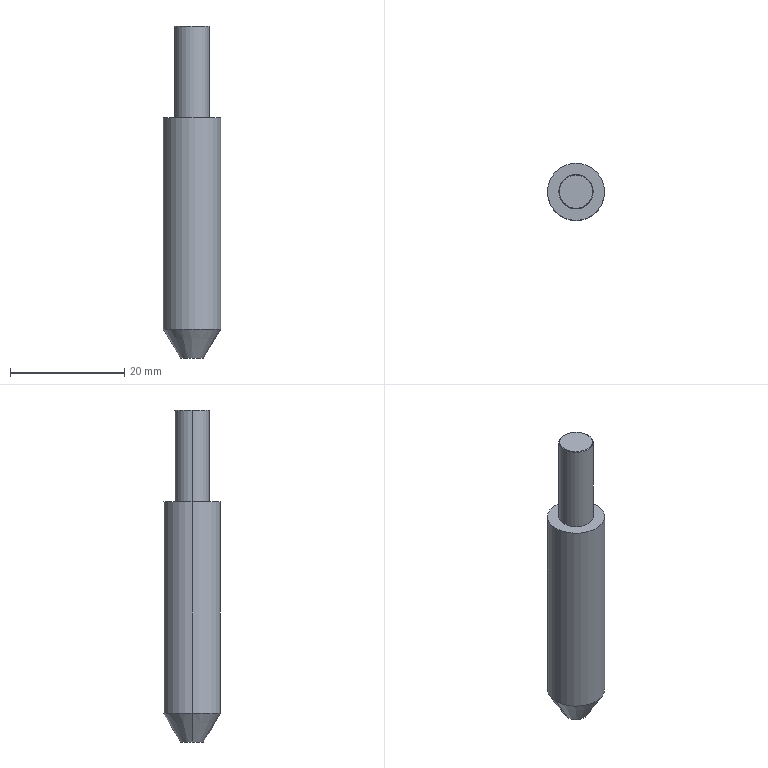Part | STEP file | Pin | 1 solid | 11 faces | box 10 x 10 x 58 mm | volume 3562 mm3 | cone 4 | cylinder 4 | plane 3 | commonest cylinder face diameters 6 x2 10 x2
STEP:
#1=CARTESIAN_POINT('',(0.,0.,0.));
#2=DIRECTION('',(0.,0.,1.));
#3=DIRECTION('',(1.,0.,0.));
#4=AXIS2_PLACEMENT_3D('',#1,#2,#3);
#5=CARTESIAN_POINT('',(-2.,0.,0.));
#6=VERTEX_POINT('',#5);
#7=CARTESIAN_POINT('',(2.,0.,0.));
#8=VERTEX_POINT('',#7);
#9=CARTESIAN_POINT('',(0.,0.,0.));
#10=DIRECTION('',(0.,0.,-1.));
#11=DIRECTION('',(1.,0.,0.));
#12=AXIS2_PLACEMENT_3D('',#9,#10,#11);
#13=CIRCLE('',#12,2.);
#14=CARTESIAN_POINT('',(0.,0.,5.));
#15=DIRECTION('',(0.,0.,1.));
#16=DIRECTION('',(1.,0.,0.));
#17=AXIS2_PLACEMENT_3D('',#14,#15,#16);
#18=CONICAL_SURFACE('',#17,5.,0.5404);
#19=CARTESIAN_POINT('',(6.283,-5.));
#20=DIRECTION('',(-1.,0.));
#21=VECTOR('',#20,1.);
#22=LINE('',#19,#21);
#23=(GEOMETRIC_REPRESENTATION_CONTEXT(2)PARAMETRIC_REPRESENTATION_CONTEXT()REPRESENTATION_CONTEXT('',''));
#24=DEFINITIONAL_REPRESENTATION('',(#22),#23);
#25=PCURVE('',#18,#24);
#26=CARTESIAN_POINT('',(0.,0.,0.));
#27=DIRECTION('',(0.,0.,1.));
#28=DIRECTION('',(1.,0.,0.));
#29=AXIS2_PLACEMENT_3D('',#26,#27,#28);
#30=PLANE('',#29);
#31=CARTESIAN_POINT('',(2.,0.));
#32=CARTESIAN_POINT('',(2.,-3.464));
#33=CARTESIAN_POINT('',(-1.,-1.732));
#34=CARTESIAN_POINT('',(-4.,0.));
#35=CARTESIAN_POINT('',(-1.,1.732));
#36=CARTESIAN_POINT('',(2.,3.464));
#37=CARTESIAN_POINT('',(2.,0.));
#38=(BOUNDED_CURVE()B_SPLINE_CURVE(2,(#31,#32,#33,#34,#35,#36,#37),.UNSPECIFIED.,.T.,.F.)B_SPLINE_CURVE_WITH_KNOTS((1,2,2,2,2,1),(-2.094,0.,2.094,4.189,6.283,8.378),.UNSPECIFIED.)CURVE()GEOMETRIC_REPRESENTATION_ITEM()RATIONAL_B_SPLINE_CURVE((1.,0.5,1.,0.5,1.,0.5,1.))REPRESENTATION_ITEM(''));
#39=(GEOMETRIC_REPRESENTATION_CONTEXT(2)PARAMETRIC_REPRESENTATION_CONTEXT()REPRESENTATION_CONTEXT('',''));
#40=DEFINITIONAL_REPRESENTATION('',(#38),#39);
#41=PCURVE('',#30,#40);
#42=SURFACE_CURVE('',#13,(#25,#41),.PCURVE_S1.);
#43=EDGE_CURVE('',#6,#8,#42,.T.);
#44=ORIENTED_EDGE('',*,*,#43,.F.);
#45=CARTESIAN_POINT('',(-5.,0.,5.));
#46=VERTEX_POINT('',#45);
#47=CARTESIAN_POINT('',(-5.,0.,5.));
#48=DIRECTION('',(-0.5145,0.,0.8575));
#49=VECTOR('',#48,1.);
#50=LINE('',#47,#49);
#51=CARTESIAN_POINT('',(3.142,0.));
#52=DIRECTION('',(0.,1.));
#53=VECTOR('',#52,1.);
#54=LINE('',#51,#53);
#55=(GEOMETRIC_REPRESENTATION_CONTEXT(2)PARAMETRIC_REPRESENTATION_CONTEXT()REPRESENTATION_CONTEXT('',''));
#56=DEFINITIONAL_REPRESENTATION('',(#54),#55);
#57=PCURVE('',#18,#56);
#58=CARTESIAN_POINT('',(0.,0.,5.));
#59=DIRECTION('',(0.,0.,1.));
#60=DIRECTION('',(1.,0.,0.));
#61=AXIS2_PLACEMENT_3D('',#58,#59,#60);
#62=CONICAL_SURFACE('',#61,5.,0.5404);
#63=CARTESIAN_POINT('',(3.142,0.));
#64=DIRECTION('',(0.,1.));
#65=VECTOR('',#64,1.);
#66=LINE('',#63,#65);
#67=(GEOMETRIC_REPRESENTATION_CONTEXT(2)PARAMETRIC_REPRESENTATION_CONTEXT()REPRESENTATION_CONTEXT('',''));
#68=DEFINITIONAL_REPRESENTATION('',(#66),#67);
#69=PCURVE('',#62,#68);
#70=SURFACE_CURVE('',#50,(#57,#69),.PCURVE_S1.);
#71=EDGE_CURVE('',#6,#46,#70,.T.);
#72=ORIENTED_EDGE('',*,*,#71,.T.);
#73=CARTESIAN_POINT('',(5.,0.,5.));
#74=VERTEX_POINT('',#73);
#75=CARTESIAN_POINT('',(0.,0.,5.));
#76=DIRECTION('',(0.,0.,1.));
#77=DIRECTION('',(1.,0.,0.));
#78=AXIS2_PLACEMENT_3D('',#75,#76,#77);
#79=CIRCLE('',#78,5.);
#80=CARTESIAN_POINT('',(0.,0.));
#81=DIRECTION('',(1.,0.));
#82=VECTOR('',#81,1.);
#83=LINE('',#80,#82);
#84=(GEOMETRIC_REPRESENTATION_CONTEXT(2)PARAMETRIC_REPRESENTATION_CONTEXT()REPRESENTATION_CONTEXT('',''));
#85=DEFINITIONAL_REPRESENTATION('',(#83),#84);
#86=PCURVE('',#18,#85);
#87=CARTESIAN_POINT('',(0.,0.,42.));
#88=DIRECTION('',(0.,0.,-1.));
#89=DIRECTION('',(-1.,0.,0.));
#90=AXIS2_PLACEMENT_3D('',#87,#88,#89);
#91=CYLINDRICAL_SURFACE('',#90,5.);
#92=CARTESIAN_POINT('',(3.142,37.));
#93=DIRECTION('',(-1.,0.));
#94=VECTOR('',#93,1.);
#95=LINE('',#92,#94);
#96=(GEOMETRIC_REPRESENTATION_CONTEXT(2)PARAMETRIC_REPRESENTATION_CONTEXT()REPRESENTATION_CONTEXT('',''));
#97=DEFINITIONAL_REPRESENTATION('',(#95),#96);
#98=PCURVE('',#91,#97);
#99=SURFACE_CURVE('',#79,(#86,#98),.PCURVE_S1.);
#100=EDGE_CURVE('',#74,#46,#99,.T.);
#101=ORIENTED_EDGE('',*,*,#100,.F.);
#102=CARTESIAN_POINT('',(5.,0.,5.));
#103=DIRECTION('',(0.5145,0.,0.8575));
#104=VECTOR('',#103,1.);
#105=LINE('',#102,#104);
#106=CARTESIAN_POINT('',(0.,0.));
#107=DIRECTION('',(0.,1.));
#108=VECTOR('',#107,1.);
#109=LINE('',#106,#108);
#110=(GEOMETRIC_REPRESENTATION_CONTEXT(2)PARAMETRIC_REPRESENTATION_CONTEXT()REPRESENTATION_CONTEXT('',''));
#111=DEFINITIONAL_REPRESENTATION('',(#109),#110);
#112=PCURVE('',#18,#111);
#113=CARTESIAN_POINT('',(6.283,0.));
#114=DIRECTION('',(0.,1.));
#115=VECTOR('',#114,1.);
#116=LINE('',#113,#115);
#117=(GEOMETRIC_REPRESENTATION_CONTEXT(2)PARAMETRIC_REPRESENTATION_CONTEXT()REPRESENTATION_CONTEXT('',''));
#118=DEFINITIONAL_REPRESENTATION('',(#116),#117);
#119=PCURVE('',#62,#118);
#120=SURFACE_CURVE('',#105,(#112,#119),.PCURVE_S1.);
#121=EDGE_CURVE('',#8,#74,#120,.T.);
#122=ORIENTED_EDGE('',*,*,#121,.F.);
#123=EDGE_LOOP('',(#44,#72,#101,#122));
#124=FACE_BOUND('',#123,.T.);
#125=ADVANCED_FACE('',(#124),#18,.T.);
#126=CARTESIAN_POINT('',(2.9,0.,58.));
#127=VERTEX_POINT('',#126);
#128=CARTESIAN_POINT('',(-2.9,0.,58.));
#129=VERTEX_POINT('',#128);
#130=CARTESIAN_POINT('',(0.,0.,58.));
#131=DIRECTION('',(0.,0.,1.));
#132=DIRECTION('',(1.,0.,0.));
#133=AXIS2_PLACEMENT_3D('',#130,#131,#132);
#134=CIRCLE('',#133,2.9);
#135=CARTESIAN_POINT('',(0.,0.,58.));
#136=DIRECTION('',(0.,0.,-1.));
#137=DIRECTION('',(-1.,0.,0.));
#138=AXIS2_PLACEMENT_3D('',#135,#136,#137);
#139=CONICAL_SURFACE('',#138,2.9,0.7854);
#140=CARTESIAN_POINT('',(3.142,0.));
#141=DIRECTION('',(-1.,0.));
#142=VECTOR('',#141,1.);
#143=LINE('',#140,#142);
#144=(GEOMETRIC_REPRESENTATION_CONTEXT(2)PARAMETRIC_REPRESENTATION_CONTEXT()REPRESENTATION_CONTEXT('',''));
#145=DEFINITIONAL_REPRESENTATION('',(#143),#144);
#146=PCURVE('',#139,#145);
#147=CARTESIAN_POINT('',(0.,0.,58.));
#148=DIRECTION('',(0.,0.,1.));
#149=DIRECTION('',(1.,0.,0.));
#150=AXIS2_PLACEMENT_3D('',#147,#148,#149);
#151=PLANE('',#150);
#152=CARTESIAN_POINT('',(0.,0.));
#153=DIRECTION('',(1.,0.));
#154=AXIS2_PLACEMENT_2D('',#152,#153);
#155=CIRCLE('',#154,2.9);
#156=(GEOMETRIC_REPRESENTATION_CONTEXT(2)PARAMETRIC_REPRESENTATION_CONTEXT()REPRESENTATION_CONTEXT('',''));
#157=DEFINITIONAL_REPRESENTATION('',(#155),#156);
#158=PCURVE('',#151,#157);
#159=SURFACE_CURVE('',#134,(#146,#158),.PCURVE_S1.);
#160=EDGE_CURVE('',#127,#129,#159,.T.);
#161=ORIENTED_EDGE('',*,*,#160,.F.);
#162=CARTESIAN_POINT('',(3.,0.,57.9));
#163=VERTEX_POINT('',#162);
#164=CARTESIAN_POINT('',(2.9,0.,58.));
#165=DIRECTION('',(0.7071,0.,-0.7071));
#166=VECTOR('',#165,1.);
#167=LINE('',#164,#166);
#168=CARTESIAN_POINT('',(3.142,0.));
#169=DIRECTION('',(0.,1.));
#170=VECTOR('',#169,1.);
#171=LINE('',#168,#170);
#172=(GEOMETRIC_REPRESENTATION_CONTEXT(2)PARAMETRIC_REPRESENTATION_CONTEXT()REPRESENTATION_CONTEXT('',''));
#173=DEFINITIONAL_REPRESENTATION('',(#171),#172);
#174=PCURVE('',#139,#173);
#175=CARTESIAN_POINT('',(0.,0.,58.));
#176=DIRECTION('',(0.,0.,-1.));
#177=DIRECTION('',(-1.,0.,0.));
#178=AXIS2_PLACEMENT_3D('',#175,#176,#177);
#179=CONICAL_SURFACE('',#178,2.9,0.7854);
#180=CARTESIAN_POINT('',(3.142,0.));
#181=DIRECTION('',(0.,1.));
#182=VECTOR('',#181,1.);
#183=LINE('',#180,#182);
#184=(GEOMETRIC_REPRESENTATION_CONTEXT(2)PARAMETRIC_REPRESENTATION_CONTEXT()REPRESENTATION_CONTEXT('',''));
#185=DEFINITIONAL_REPRESENTATION('',(#183),#184);
#186=PCURVE('',#179,#185);
#187=SURFACE_CURVE('',#167,(#174,#186),.PCURVE_S1.);
#188=EDGE_CURVE('',#127,#163,#187,.T.);
#189=ORIENTED_EDGE('',*,*,#188,.T.);
#190=CARTESIAN_POINT('',(-3.,0.,57.9));
#191=VERTEX_POINT('',#190);
#192=CARTESIAN_POINT('',(0.,0.,57.9));
#193=DIRECTION('',(0.,0.,-1.));
#194=DIRECTION('',(1.,0.,0.));
#195=AXIS2_PLACEMENT_3D('',#192,#193,#194);
#196=CIRCLE('',#195,3.);
#197=CARTESIAN_POINT('',(-3.142,0.1));
#198=DIRECTION('',(1.,0.));
#199=VECTOR('',#198,1.);
#200=LINE('',#197,#199);
#201=(GEOMETRIC_REPRESENTATION_CONTEXT(2)PARAMETRIC_REPRESENTATION_CONTEXT()REPRESENTATION_CONTEXT('',''));
#202=DEFINITIONAL_REPRESENTATION('',(#200),#201);
#203=PCURVE('',#139,#202);
#204=CARTESIAN_POINT('',(0.,0.,58.));
#205=DIRECTION('',(0.,0.,-1.));
#206=DIRECTION('',(-1.,0.,0.));
#207=AXIS2_PLACEMENT_3D('',#204,#205,#206);
#208=CYLINDRICAL_SURFACE('',#207,3.);
#209=CARTESIAN_POINT('',(-3.142,0.1));
#210=DIRECTION('',(1.,0.));
#211=VECTOR('',#210,1.);
#212=LINE('',#209,#211);
#213=(GEOMETRIC_REPRESENTATION_CONTEXT(2)PARAMETRIC_REPRESENTATION_CONTEXT()REPRESENTATION_CONTEXT('',''));
#214=DEFINITIONAL_REPRESENTATION('',(#212),#213);
#215=PCURVE('',#208,#214);
#216=SURFACE_CURVE('',#196,(#203,#215),.PCURVE_S1.);
#217=EDGE_CURVE('',#191,#163,#216,.T.);
#218=ORIENTED_EDGE('',*,*,#217,.F.);
#219=CARTESIAN_POINT('',(-2.9,0.,58.));
#220=DIRECTION('',(-0.7071,0.,-0.7071));
#221=VECTOR('',#220,1.);
#222=LINE('',#219,#221);
#223=CARTESIAN_POINT('',(0.,0.));
#224=DIRECTION('',(0.,1.));
#225=VECTOR('',#224,1.);
#226=LINE('',#223,#225);
#227=(GEOMETRIC_REPRESENTATION_CONTEXT(2)PARAMETRIC_REPRESENTATION_CONTEXT()REPRESENTATION_CONTEXT('',''));
#228=DEFINITIONAL_REPRESENTATION('',(#226),#227);
#229=PCURVE('',#139,#228);
#230=CARTESIAN_POINT('',(6.283,0.));
#231=DIRECTION('',(0.,1.));
#232=VECTOR('',#231,1.);
#233=LINE('',#230,#232);
#234=(GEOMETRIC_REPRESENTATION_CONTEXT(2)PARAMETRIC_REPRESENTATION_CONTEXT()REPRESENTATION_CONTEXT('',''));
#235=DEFINITIONAL_REPRESENTATION('',(#233),#234);
#236=PCURVE('',#179,#235);
#237=SURFACE_CURVE('',#222,(#229,#236),.PCURVE_S1.);
#238=EDGE_CURVE('',#129,#191,#237,.T.);
#239=ORIENTED_EDGE('',*,*,#238,.F.);
#240=EDGE_LOOP('',(#161,#189,#218,#239));
#241=FACE_BOUND('',#240,.T.);
#242=ADVANCED_FACE('',(#241),#139,.T.);
#243=ORIENTED_EDGE('',*,*,#217,.T.);
#244=CARTESIAN_POINT('',(3.,0.,42.));
#245=VERTEX_POINT('',#244);
#246=CARTESIAN_POINT('',(3.,0.,58.));
#247=DIRECTION('',(0.,0.,-1.));
#248=VECTOR('',#247,1.);
#249=LINE('',#246,#248);
#250=CARTESIAN_POINT('',(3.142,0.));
#251=DIRECTION('',(0.,1.));
#252=VECTOR('',#251,1.);
#253=LINE('',#250,#252);
#254=(GEOMETRIC_REPRESENTATION_CONTEXT(2)PARAMETRIC_REPRESENTATION_CONTEXT()REPRESENTATION_CONTEXT('',''));
#255=DEFINITIONAL_REPRESENTATION('',(#253),#254);
#256=PCURVE('',#208,#255);
#257=CARTESIAN_POINT('',(0.,0.,58.));
#258=DIRECTION('',(0.,0.,-1.));
#259=DIRECTION('',(-1.,0.,0.));
#260=AXIS2_PLACEMENT_3D('',#257,#258,#259);
#261=CYLINDRICAL_SURFACE('',#260,3.);
#262=CARTESIAN_POINT('',(3.142,0.));
#263=DIRECTION('',(0.,1.));
#264=VECTOR('',#263,1.);
#265=LINE('',#262,#264);
#266=(GEOMETRIC_REPRESENTATION_CONTEXT(2)PARAMETRIC_REPRESENTATION_CONTEXT()REPRESENTATION_CONTEXT('',''));
#267=DEFINITIONAL_REPRESENTATION('',(#265),#266);
#268=PCURVE('',#261,#267);
#269=SURFACE_CURVE('',#249,(#256,#268),.PCURVE_S1.);
#270=EDGE_CURVE('',#163,#245,#269,.T.);
#271=ORIENTED_EDGE('',*,*,#270,.T.);
#272=CARTESIAN_POINT('',(-3.,0.,42.));
#273=VERTEX_POINT('',#272);
#274=CARTESIAN_POINT('',(0.,0.,42.));
#275=DIRECTION('',(0.,0.,1.));
#276=DIRECTION('',(1.,0.,0.));
#277=AXIS2_PLACEMENT_3D('',#274,#275,#276);
#278=CIRCLE('',#277,3.);
#279=CARTESIAN_POINT('',(3.142,16.));
#280=DIRECTION('',(-1.,0.));
#281=VECTOR('',#280,1.);
#282=LINE('',#279,#281);
#283=(GEOMETRIC_REPRESENTATION_CONTEXT(2)PARAMETRIC_REPRESENTATION_CONTEXT()REPRESENTATION_CONTEXT('',''));
#284=DEFINITIONAL_REPRESENTATION('',(#282),#283);
#285=PCURVE('',#208,#284);
#286=CARTESIAN_POINT('',(0.,0.,42.));
#287=DIRECTION('',(0.,0.,1.));
#288=DIRECTION('',(1.,0.,0.));
#289=AXIS2_PLACEMENT_3D('',#286,#287,#288);
#290=PLANE('',#289);
#291=CARTESIAN_POINT('',(0.,0.));
#292=DIRECTION('',(1.,0.));
#293=AXIS2_PLACEMENT_2D('',#291,#292);
#294=CIRCLE('',#293,3.);
#295=(GEOMETRIC_REPRESENTATION_CONTEXT(2)PARAMETRIC_REPRESENTATION_CONTEXT()REPRESENTATION_CONTEXT('',''));
#296=DEFINITIONAL_REPRESENTATION('',(#294),#295);
#297=PCURVE('',#290,#296);
#298=SURFACE_CURVE('',#278,(#285,#297),.PCURVE_S1.);
#299=EDGE_CURVE('',#245,#273,#298,.T.);
#300=ORIENTED_EDGE('',*,*,#299,.T.);
#301=CARTESIAN_POINT('',(-3.,0.,58.));
#302=DIRECTION('',(0.,0.,-1.));
#303=VECTOR('',#302,1.);
#304=LINE('',#301,#303);
#305=CARTESIAN_POINT('',(0.,0.));
#306=DIRECTION('',(0.,1.));
#307=VECTOR('',#306,1.);
#308=LINE('',#305,#307);
#309=(GEOMETRIC_REPRESENTATION_CONTEXT(2)PARAMETRIC_REPRESENTATION_CONTEXT()REPRESENTATION_CONTEXT('',''));
#310=DEFINITIONAL_REPRESENTATION('',(#308),#309);
#311=PCURVE('',#208,#310);
#312=CARTESIAN_POINT('',(6.283,0.));
#313=DIRECTION('',(0.,1.));
#314=VECTOR('',#313,1.);
#315=LINE('',#312,#314);
#316=(GEOMETRIC_REPRESENTATION_CONTEXT(2)PARAMETRIC_REPRESENTATION_CONTEXT()REPRESENTATION_CONTEXT('',''));
#317=DEFINITIONAL_REPRESENTATION('',(#315),#316);
#318=PCURVE('',#261,#317);
#319=SURFACE_CURVE('',#304,(#311,#318),.PCURVE_S1.);
#320=EDGE_CURVE('',#191,#273,#319,.T.);
#321=ORIENTED_EDGE('',*,*,#320,.F.);
#322=EDGE_LOOP('',(#243,#271,#300,#321));
#323=FACE_BOUND('',#322,.T.);
#324=ADVANCED_FACE('',(#323),#208,.T.);
#325=CARTESIAN_POINT('',(5.,0.,42.));
#326=VERTEX_POINT('',#325);
#327=CARTESIAN_POINT('',(-5.,0.,42.));
#328=VERTEX_POINT('',#327);
#329=CARTESIAN_POINT('',(0.,0.,42.));
#330=DIRECTION('',(0.,0.,1.));
#331=DIRECTION('',(1.,0.,0.));
#332=AXIS2_PLACEMENT_3D('',#329,#330,#331);
#333=CIRCLE('',#332,5.);
#334=CARTESIAN_POINT('',(3.142,0.));
#335=DIRECTION('',(-1.,0.));
#336=VECTOR('',#335,1.);
#337=LINE('',#334,#336);
#338=(GEOMETRIC_REPRESENTATION_CONTEXT(2)PARAMETRIC_REPRESENTATION_CONTEXT()REPRESENTATION_CONTEXT('',''));
#339=DEFINITIONAL_REPRESENTATION('',(#337),#338);
#340=PCURVE('',#91,#339);
#341=CARTESIAN_POINT('',(0.,0.));
#342=DIRECTION('',(1.,0.));
#343=AXIS2_PLACEMENT_2D('',#341,#342);
#344=CIRCLE('',#343,5.);
#345=(GEOMETRIC_REPRESENTATION_CONTEXT(2)PARAMETRIC_REPRESENTATION_CONTEXT()REPRESENTATION_CONTEXT('',''));
#346=DEFINITIONAL_REPRESENTATION('',(#344),#345);
#347=PCURVE('',#290,#346);
#348=SURFACE_CURVE('',#333,(#340,#347),.PCURVE_S1.);
#349=EDGE_CURVE('',#326,#328,#348,.T.);
#350=ORIENTED_EDGE('',*,*,#349,.F.);
#351=CARTESIAN_POINT('',(5.,0.,42.));
#352=DIRECTION('',(0.,0.,-1.));
#353=VECTOR('',#352,1.);
#354=LINE('',#351,#353);
#355=CARTESIAN_POINT('',(3.142,0.));
#356=DIRECTION('',(0.,1.));
#357=VECTOR('',#356,1.);
#358=LINE('',#355,#357);
#359=(GEOMETRIC_REPRESENTATION_CONTEXT(2)PARAMETRIC_REPRESENTATION_CONTEXT()REPRESENTATION_CONTEXT('',''));
#360=DEFINITIONAL_REPRESENTATION('',(#358),#359);
#361=PCURVE('',#91,#360);
#362=CARTESIAN_POINT('',(0.,0.,42.));
#363=DIRECTION('',(0.,0.,-1.));
#364=DIRECTION('',(-1.,0.,0.));
#365=AXIS2_PLACEMENT_3D('',#362,#363,#364);
#366=CYLINDRICAL_SURFACE('',#365,5.);
#367=CARTESIAN_POINT('',(3.142,0.));
#368=DIRECTION('',(0.,1.));
#369=VECTOR('',#368,1.);
#370=LINE('',#367,#369);
#371=(GEOMETRIC_REPRESENTATION_CONTEXT(2)PARAMETRIC_REPRESENTATION_CONTEXT()REPRESENTATION_CONTEXT('',''));
#372=DEFINITIONAL_REPRESENTATION('',(#370),#371);
#373=PCURVE('',#366,#372);
#374=SURFACE_CURVE('',#354,(#361,#373),.PCURVE_S1.);
#375=EDGE_CURVE('',#326,#74,#374,.T.);
#376=ORIENTED_EDGE('',*,*,#375,.T.);
#377=ORIENTED_EDGE('',*,*,#100,.T.);
#378=CARTESIAN_POINT('',(-5.,0.,42.));
#379=DIRECTION('',(0.,0.,-1.));
#380=VECTOR('',#379,1.);
#381=LINE('',#378,#380);
#382=CARTESIAN_POINT('',(0.,0.));
#383=DIRECTION('',(0.,1.));
#384=VECTOR('',#383,1.);
#385=LINE('',#382,#384);
#386=(GEOMETRIC_REPRESENTATION_CONTEXT(2)PARAMETRIC_REPRESENTATION_CONTEXT()REPRESENTATION_CONTEXT('',''));
#387=DEFINITIONAL_REPRESENTATION('',(#385),#386);
#388=PCURVE('',#91,#387);
#389=CARTESIAN_POINT('',(6.283,0.));
#390=DIRECTION('',(0.,1.));
#391=VECTOR('',#390,1.);
#392=LINE('',#389,#391);
#393=(GEOMETRIC_REPRESENTATION_CONTEXT(2)PARAMETRIC_REPRESENTATION_CONTEXT()REPRESENTATION_CONTEXT('',''));
#394=DEFINITIONAL_REPRESENTATION('',(#392),#393);
#395=PCURVE('',#366,#394);
#396=SURFACE_CURVE('',#381,(#388,#395),.PCURVE_S1.);
#397=EDGE_CURVE('',#328,#46,#396,.T.);
#398=ORIENTED_EDGE('',*,*,#397,.F.);
#399=EDGE_LOOP('',(#350,#376,#377,#398));
#400=FACE_BOUND('',#399,.T.);
#401=ADVANCED_FACE('',(#400),#91,.T.);
#402=CARTESIAN_POINT('',(0.,0.,42.));
#403=DIRECTION('',(0.,0.,1.));
#404=DIRECTION('',(1.,0.,0.));
#405=AXIS2_PLACEMENT_3D('',#402,#403,#404);
#406=CIRCLE('',#405,5.);
#407=CARTESIAN_POINT('',(0.,0.));
#408=DIRECTION('',(1.,0.));
#409=AXIS2_PLACEMENT_2D('',#407,#408);
#410=CIRCLE('',#409,5.);
#411=(GEOMETRIC_REPRESENTATION_CONTEXT(2)PARAMETRIC_REPRESENTATION_CONTEXT()REPRESENTATION_CONTEXT('',''));
#412=DEFINITIONAL_REPRESENTATION('',(#410),#411);
#413=PCURVE('',#290,#412);
#414=CARTESIAN_POINT('',(9.425,0.));
#415=DIRECTION('',(-1.,0.));
#416=VECTOR('',#415,1.);
#417=LINE('',#414,#416);
#418=(GEOMETRIC_REPRESENTATION_CONTEXT(2)PARAMETRIC_REPRESENTATION_CONTEXT()REPRESENTATION_CONTEXT('',''));
#419=DEFINITIONAL_REPRESENTATION('',(#417),#418);
#420=PCURVE('',#366,#419);
#421=SURFACE_CURVE('',#406,(#413,#420),.PCURVE_S1.);
#422=EDGE_CURVE('',#328,#326,#421,.T.);
#423=ORIENTED_EDGE('',*,*,#422,.T.);
#424=ORIENTED_EDGE('',*,*,#349,.T.);
#425=EDGE_LOOP('',(#423,#424));
#426=FACE_BOUND('',#425,.T.);
#427=CARTESIAN_POINT('',(0.,0.,42.));
#428=DIRECTION('',(0.,0.,1.));
#429=DIRECTION('',(1.,0.,0.));
#430=AXIS2_PLACEMENT_3D('',#427,#428,#429);
#431=CIRCLE('',#430,3.);
#432=CARTESIAN_POINT('',(0.,0.));
#433=DIRECTION('',(1.,0.));
#434=AXIS2_PLACEMENT_2D('',#432,#433);
#435=CIRCLE('',#434,3.);
#436=(GEOMETRIC_REPRESENTATION_CONTEXT(2)PARAMETRIC_REPRESENTATION_CONTEXT()REPRESENTATION_CONTEXT('',''));
#437=DEFINITIONAL_REPRESENTATION('',(#435),#436);
#438=PCURVE('',#290,#437);
#439=CARTESIAN_POINT('',(9.425,16.));
#440=DIRECTION('',(-1.,0.));
#441=VECTOR('',#440,1.);
#442=LINE('',#439,#441);
#443=(GEOMETRIC_REPRESENTATION_CONTEXT(2)PARAMETRIC_REPRESENTATION_CONTEXT()REPRESENTATION_CONTEXT('',''));
#444=DEFINITIONAL_REPRESENTATION('',(#442),#443);
#445=PCURVE('',#261,#444);
#446=SURFACE_CURVE('',#431,(#438,#445),.PCURVE_S1.);
#447=EDGE_CURVE('',#273,#245,#446,.T.);
#448=ORIENTED_EDGE('',*,*,#447,.F.);
#449=ORIENTED_EDGE('',*,*,#299,.F.);
#450=EDGE_LOOP('',(#448,#449));
#451=FACE_BOUND('',#450,.T.);
#452=ADVANCED_FACE('',(#426,#451),#290,.T.);
#453=ORIENTED_EDGE('',*,*,#375,.F.);
#454=ORIENTED_EDGE('',*,*,#422,.F.);
#455=ORIENTED_EDGE('',*,*,#397,.T.);
#456=CARTESIAN_POINT('',(0.,0.,5.));
#457=DIRECTION('',(0.,0.,1.));
#458=DIRECTION('',(1.,0.,0.));
#459=AXIS2_PLACEMENT_3D('',#456,#457,#458);
#460=CIRCLE('',#459,5.);
#461=CARTESIAN_POINT('',(9.425,37.));
#462=DIRECTION('',(-1.,0.));
#463=VECTOR('',#462,1.);
#464=LINE('',#461,#463);
#465=(GEOMETRIC_REPRESENTATION_CONTEXT(2)PARAMETRIC_REPRESENTATION_CONTEXT()REPRESENTATION_CONTEXT('',''));
#466=DEFINITIONAL_REPRESENTATION('',(#464),#465);
#467=PCURVE('',#366,#466);
#468=CARTESIAN_POINT('',(0.,0.));
#469=DIRECTION('',(1.,0.));
#470=VECTOR('',#469,1.);
#471=LINE('',#468,#470);
#472=(GEOMETRIC_REPRESENTATION_CONTEXT(2)PARAMETRIC_REPRESENTATION_CONTEXT()REPRESENTATION_CONTEXT('',''));
#473=DEFINITIONAL_REPRESENTATION('',(#471),#472);
#474=PCURVE('',#62,#473);
#475=SURFACE_CURVE('',#460,(#467,#474),.PCURVE_S1.);
#476=EDGE_CURVE('',#46,#74,#475,.T.);
#477=ORIENTED_EDGE('',*,*,#476,.T.);
#478=EDGE_LOOP('',(#453,#454,#455,#477));
#479=FACE_BOUND('',#478,.T.);
#480=ADVANCED_FACE('',(#479),#366,.T.);
#481=CARTESIAN_POINT('',(0.,0.,0.));
#482=DIRECTION('',(0.,0.,-1.));
#483=DIRECTION('',(1.,0.,0.));
#484=AXIS2_PLACEMENT_3D('',#481,#482,#483);
#485=CIRCLE('',#484,2.);
#486=CARTESIAN_POINT('',(2.,0.));
#487=CARTESIAN_POINT('',(2.,-3.464));
#488=CARTESIAN_POINT('',(-1.,-1.732));
#489=CARTESIAN_POINT('',(-4.,0.));
#490=CARTESIAN_POINT('',(-1.,1.732));
#491=CARTESIAN_POINT('',(2.,3.464));
#492=CARTESIAN_POINT('',(2.,0.));
#493=(BOUNDED_CURVE()B_SPLINE_CURVE(2,(#486,#487,#488,#489,#490,#491,#492),.UNSPECIFIED.,.T.,.F.)B_SPLINE_CURVE_WITH_KNOTS((1,2,2,2,2,1),(-2.094,0.,2.094,4.189,6.283,8.378),.UNSPECIFIED.)CURVE()GEOMETRIC_REPRESENTATION_ITEM()RATIONAL_B_SPLINE_CURVE((1.,0.5,1.,0.5,1.,0.5,1.))REPRESENTATION_ITEM(''));
#494=(GEOMETRIC_REPRESENTATION_CONTEXT(2)PARAMETRIC_REPRESENTATION_CONTEXT()REPRESENTATION_CONTEXT('',''));
#495=DEFINITIONAL_REPRESENTATION('',(#493),#494);
#496=PCURVE('',#30,#495);
#497=CARTESIAN_POINT('',(6.283,-5.));
#498=DIRECTION('',(-1.,0.));
#499=VECTOR('',#498,1.);
#500=LINE('',#497,#499);
#501=(GEOMETRIC_REPRESENTATION_CONTEXT(2)PARAMETRIC_REPRESENTATION_CONTEXT()REPRESENTATION_CONTEXT('',''));
#502=DEFINITIONAL_REPRESENTATION('',(#500),#501);
#503=PCURVE('',#62,#502);
#504=SURFACE_CURVE('',#485,(#496,#503),.PCURVE_S1.);
#505=EDGE_CURVE('',#8,#6,#504,.T.);
#506=ORIENTED_EDGE('',*,*,#505,.T.);
#507=ORIENTED_EDGE('',*,*,#43,.T.);
#508=EDGE_LOOP('',(#506,#507));
#509=FACE_BOUND('',#508,.T.);
#510=ADVANCED_FACE('',(#509),#30,.F.);
#511=ORIENTED_EDGE('',*,*,#270,.F.);
#512=CARTESIAN_POINT('',(0.,0.,57.9));
#513=DIRECTION('',(0.,0.,-1.));
#514=DIRECTION('',(1.,0.,0.));
#515=AXIS2_PLACEMENT_3D('',#512,#513,#514);
#516=CIRCLE('',#515,3.);
#517=CARTESIAN_POINT('',(3.142,0.1));
#518=DIRECTION('',(1.,0.));
#519=VECTOR('',#518,1.);
#520=LINE('',#517,#519);
#521=(GEOMETRIC_REPRESENTATION_CONTEXT(2)PARAMETRIC_REPRESENTATION_CONTEXT()REPRESENTATION_CONTEXT('',''));
#522=DEFINITIONAL_REPRESENTATION('',(#520),#521);
#523=PCURVE('',#261,#522);
#524=CARTESIAN_POINT('',(3.142,0.1));
#525=DIRECTION('',(1.,0.));
#526=VECTOR('',#525,1.);
#527=LINE('',#524,#526);
#528=(GEOMETRIC_REPRESENTATION_CONTEXT(2)PARAMETRIC_REPRESENTATION_CONTEXT()REPRESENTATION_CONTEXT('',''));
#529=DEFINITIONAL_REPRESENTATION('',(#527),#528);
#530=PCURVE('',#179,#529);
#531=SURFACE_CURVE('',#516,(#523,#530),.PCURVE_S1.);
#532=EDGE_CURVE('',#163,#191,#531,.T.);
#533=ORIENTED_EDGE('',*,*,#532,.T.);
#534=ORIENTED_EDGE('',*,*,#320,.T.);
#535=ORIENTED_EDGE('',*,*,#447,.T.);
#536=EDGE_LOOP('',(#511,#533,#534,#535));
#537=FACE_BOUND('',#536,.T.);
#538=ADVANCED_FACE('',(#537),#261,.T.);
#539=CARTESIAN_POINT('',(0.,0.,58.));
#540=DIRECTION('',(0.,0.,1.));
#541=DIRECTION('',(1.,0.,0.));
#542=AXIS2_PLACEMENT_3D('',#539,#540,#541);
#543=CIRCLE('',#542,2.9);
#544=CARTESIAN_POINT('',(0.,0.));
#545=DIRECTION('',(1.,0.));
#546=AXIS2_PLACEMENT_2D('',#544,#545);
#547=CIRCLE('',#546,2.9);
#548=(GEOMETRIC_REPRESENTATION_CONTEXT(2)PARAMETRIC_REPRESENTATION_CONTEXT()REPRESENTATION_CONTEXT('',''));
#549=DEFINITIONAL_REPRESENTATION('',(#547),#548);
#550=PCURVE('',#151,#549);
#551=CARTESIAN_POINT('',(9.425,0.));
#552=DIRECTION('',(-1.,0.));
#553=VECTOR('',#552,1.);
#554=LINE('',#551,#553);
#555=(GEOMETRIC_REPRESENTATION_CONTEXT(2)PARAMETRIC_REPRESENTATION_CONTEXT()REPRESENTATION_CONTEXT('',''));
#556=DEFINITIONAL_REPRESENTATION('',(#554),#555);
#557=PCURVE('',#179,#556);
#558=SURFACE_CURVE('',#543,(#550,#557),.PCURVE_S1.);
#559=EDGE_CURVE('',#129,#127,#558,.T.);
#560=ORIENTED_EDGE('',*,*,#559,.T.);
#561=ORIENTED_EDGE('',*,*,#160,.T.);
#562=EDGE_LOOP('',(#560,#561));
#563=FACE_BOUND('',#562,.T.);
#564=ADVANCED_FACE('',(#563),#151,.T.);
#565=ORIENTED_EDGE('',*,*,#188,.F.);
#566=ORIENTED_EDGE('',*,*,#559,.F.);
#567=ORIENTED_EDGE('',*,*,#238,.T.);
#568=ORIENTED_EDGE('',*,*,#532,.F.);
#569=EDGE_LOOP('',(#565,#566,#567,#568));
#570=FACE_BOUND('',#569,.T.);
#571=ADVANCED_FACE('',(#570),#179,.T.);
#572=ORIENTED_EDGE('',*,*,#71,.F.);
#573=ORIENTED_EDGE('',*,*,#505,.F.);
#574=ORIENTED_EDGE('',*,*,#121,.T.);
#575=ORIENTED_EDGE('',*,*,#476,.F.);
#576=EDGE_LOOP('',(#572,#573,#574,#575));
#577=FACE_BOUND('',#576,.T.);
#578=ADVANCED_FACE('',(#577),#62,.T.);
#579=CLOSED_SHELL('',(#125,#242,#324,#401,#452,#480,#510,#538,#564,#571,#578));
#580=MANIFOLD_SOLID_BREP('',#579);
#581=(LENGTH_UNIT()NAMED_UNIT(*)SI_UNIT(.MILLI.,.METRE.));
#582=UNCERTAINTY_MEASURE_WITH_UNIT(LENGTH_MEASURE(0.0000001),#581,'','');
#583=(NAMED_UNIT(*)PLANE_ANGLE_UNIT()SI_UNIT($,.RADIAN.));
#584=(NAMED_UNIT(*)SI_UNIT($,.STERADIAN.)SOLID_ANGLE_UNIT());
#585=(GEOMETRIC_REPRESENTATION_CONTEXT(3)GLOBAL_UNCERTAINTY_ASSIGNED_CONTEXT((#582))GLOBAL_UNIT_ASSIGNED_CONTEXT((#581,#583,#584))REPRESENTATION_CONTEXT('',''));
#586=ADVANCED_BREP_SHAPE_REPRESENTATION('',(#4,#580),#585);